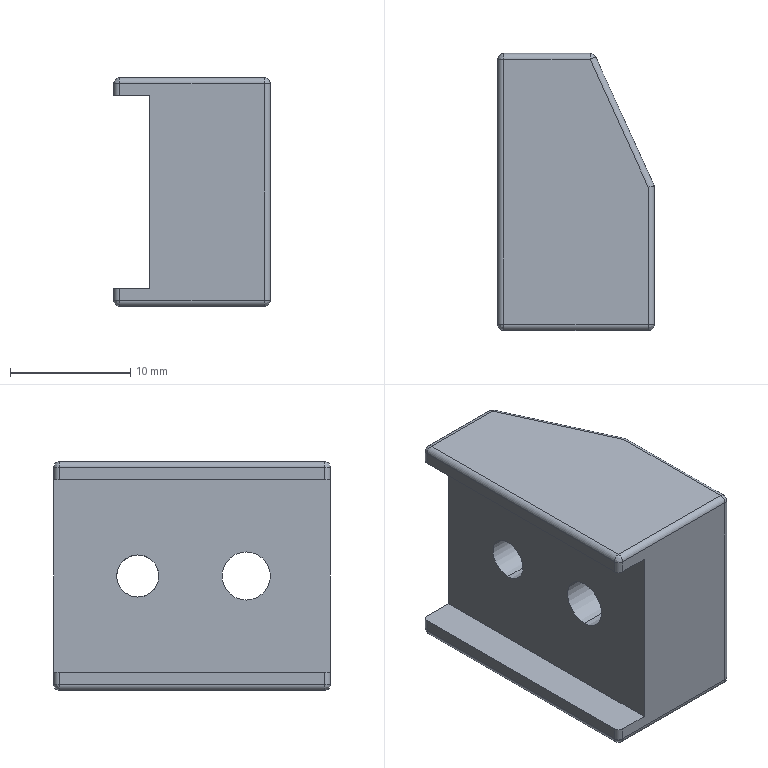Part | STEP file | Guide wheel mechanism revised.sldasm-Part-506 | 1 solid | 39 faces | box 13 x 23 x 19 mm | volume 3841 mm3 | cylinder 20 | plane 11 | spline 8 | commonest cylinder face diameters 1 x16 3.5 x2 4 x2
STEP:
#1=CARTESIAN_POINT('',(-1.818,9.,-1.75));
#2=VERTEX_POINT('',#1);
#3=CARTESIAN_POINT('',(-1.818,9.,1.75));
#4=VERTEX_POINT('',#3);
#5=CARTESIAN_POINT('',(-1.818,9.,-1.75));
#6=CARTESIAN_POINT('',(-0.2273,5.5,-1.75));
#7=CARTESIAN_POINT('',(-0.2273,5.5,1.75));
#8=CARTESIAN_POINT('',(-1.818,9.,1.75));
#9=(BOUNDED_CURVE()B_SPLINE_CURVE(3,(#5,#6,#7,#8),.UNSPECIFIED.,.F.,.F.)B_SPLINE_CURVE_WITH_KNOTS((4,4),(1.571,4.712),.UNSPECIFIED.)CURVE()GEOMETRIC_REPRESENTATION_ITEM()RATIONAL_B_SPLINE_CURVE((1.,0.3333,0.3333,1.))REPRESENTATION_ITEM(''));
#10=EDGE_CURVE('',#2,#4,#9,.T.);
#11=ORIENTED_EDGE('',*,*,#10,.F.);
#12=CARTESIAN_POINT('',(-10.,9.,-1.75));
#13=VERTEX_POINT('',#12);
#14=CARTESIAN_POINT('',(1.865,9.,-1.75));
#15=DIRECTION('',(-1.,0.,0.));
#16=VECTOR('',#15,1000.);
#17=LINE('',#14,#16);
#18=EDGE_CURVE('',#2,#13,#17,.T.);
#19=ORIENTED_EDGE('',*,*,#18,.T.);
#20=CARTESIAN_POINT('',(-10.,9.,1.75));
#21=VERTEX_POINT('',#20);
#22=CARTESIAN_POINT('',(-10.,9.,0.));
#23=DIRECTION('',(-1.,0.,0.));
#24=DIRECTION('',(0.,0.,1.));
#25=AXIS2_PLACEMENT_3D('',#22,#23,#24);
#26=CIRCLE('',#25,1.75);
#27=EDGE_CURVE('',#13,#21,#26,.T.);
#28=ORIENTED_EDGE('',*,*,#27,.T.);
#29=CARTESIAN_POINT('',(1.865,9.,1.75));
#30=DIRECTION('',(-1.,0.,0.));
#31=VECTOR('',#30,1000.);
#32=LINE('',#29,#31);
#33=EDGE_CURVE('',#4,#21,#32,.T.);
#34=ORIENTED_EDGE('',*,*,#33,.F.);
#35=EDGE_LOOP('',(#11,#19,#28,#34));
#36=FACE_OUTER_BOUND('',#35,.T.);
#37=CARTESIAN_POINT('',(1.865,9.,0.));
#38=DIRECTION('',(-1.,0.,0.));
#39=DIRECTION('',(0.,0.,1.));
#40=AXIS2_PLACEMENT_3D('',#37,#38,#39);
#41=CYLINDRICAL_SURFACE('',#40,1.75);
#42=ADVANCED_FACE('',(#36),#41,.F.);
#43=CARTESIAN_POINT('',(0.,0.,-2.));
#44=VERTEX_POINT('',#43);
#45=CARTESIAN_POINT('',(0.,0.,2.));
#46=VERTEX_POINT('',#45);
#47=CARTESIAN_POINT('',(0.,0.,0.));
#48=DIRECTION('',(-1.,0.,0.));
#49=DIRECTION('',(0.,0.,1.));
#50=AXIS2_PLACEMENT_3D('',#47,#48,#49);
#51=CIRCLE('',#50,2.);
#52=EDGE_CURVE('',#44,#46,#51,.T.);
#53=ORIENTED_EDGE('',*,*,#52,.F.);
#54=CARTESIAN_POINT('',(-10.,0.,-2.));
#55=VERTEX_POINT('',#54);
#56=CARTESIAN_POINT('',(0.,0.,-2.));
#57=DIRECTION('',(-1.,0.,0.));
#58=VECTOR('',#57,1000.);
#59=LINE('',#56,#58);
#60=EDGE_CURVE('',#44,#55,#59,.T.);
#61=ORIENTED_EDGE('',*,*,#60,.T.);
#62=CARTESIAN_POINT('',(-10.,0.,2.));
#63=VERTEX_POINT('',#62);
#64=CARTESIAN_POINT('',(-10.,0.,0.));
#65=DIRECTION('',(-1.,0.,0.));
#66=DIRECTION('',(0.,0.,1.));
#67=AXIS2_PLACEMENT_3D('',#64,#65,#66);
#68=CIRCLE('',#67,2.);
#69=EDGE_CURVE('',#55,#63,#68,.T.);
#70=ORIENTED_EDGE('',*,*,#69,.T.);
#71=CARTESIAN_POINT('',(0.,0.,2.));
#72=DIRECTION('',(-1.,0.,0.));
#73=VECTOR('',#72,1000.);
#74=LINE('',#71,#73);
#75=EDGE_CURVE('',#46,#63,#74,.T.);
#76=ORIENTED_EDGE('',*,*,#75,.F.);
#77=EDGE_LOOP('',(#53,#61,#70,#76));
#78=FACE_OUTER_BOUND('',#77,.T.);
#79=CARTESIAN_POINT('',(0.,0.,0.));
#80=DIRECTION('',(-1.,0.,0.));
#81=DIRECTION('',(0.,0.,1.));
#82=AXIS2_PLACEMENT_3D('',#79,#80,#81);
#83=CYLINDRICAL_SURFACE('',#82,2.);
#84=ADVANCED_FACE('',(#78),#83,.F.);
#85=CARTESIAN_POINT('',(-10.,9.,0.));
#86=DIRECTION('',(-1.,0.,0.));
#87=DIRECTION('',(0.,0.,1.));
#88=AXIS2_PLACEMENT_3D('',#85,#86,#87);
#89=CIRCLE('',#88,1.75);
#90=EDGE_CURVE('',#21,#13,#89,.T.);
#91=ORIENTED_EDGE('',*,*,#90,.F.);
#92=ORIENTED_EDGE('',*,*,#27,.F.);
#93=EDGE_LOOP('',(#91,#92));
#94=FACE_BOUND('',#93,.T.);
#95=CARTESIAN_POINT('',(-10.,0.,0.));
#96=DIRECTION('',(-1.,0.,0.));
#97=DIRECTION('',(0.,0.,1.));
#98=AXIS2_PLACEMENT_3D('',#95,#96,#97);
#99=CIRCLE('',#98,2.);
#100=EDGE_CURVE('',#63,#55,#99,.T.);
#101=ORIENTED_EDGE('',*,*,#100,.F.);
#102=ORIENTED_EDGE('',*,*,#69,.F.);
#103=EDGE_LOOP('',(#101,#102));
#104=FACE_BOUND('',#103,.T.);
#105=CARTESIAN_POINT('',(-10.,16.,-8.));
#106=VERTEX_POINT('',#105);
#107=CARTESIAN_POINT('',(-10.,16.,8.));
#108=VERTEX_POINT('',#107);
#109=CARTESIAN_POINT('',(-10.,16.,-8.));
#110=DIRECTION('',(0.,0.,1.));
#111=VECTOR('',#110,1000.);
#112=LINE('',#109,#111);
#113=EDGE_CURVE('',#106,#108,#112,.T.);
#114=ORIENTED_EDGE('',*,*,#113,.F.);
#115=CARTESIAN_POINT('',(-10.,-7.,-8.));
#116=VERTEX_POINT('',#115);
#117=CARTESIAN_POINT('',(-10.,-7.,-8.));
#118=DIRECTION('',(0.,1.,0.));
#119=VECTOR('',#118,1000.);
#120=LINE('',#117,#119);
#121=EDGE_CURVE('',#116,#106,#120,.T.);
#122=ORIENTED_EDGE('',*,*,#121,.F.);
#123=CARTESIAN_POINT('',(-10.,-7.,8.));
#124=VERTEX_POINT('',#123);
#125=CARTESIAN_POINT('',(-10.,-7.,-8.));
#126=DIRECTION('',(0.,0.,-1.));
#127=VECTOR('',#126,1000.);
#128=LINE('',#125,#127);
#129=EDGE_CURVE('',#124,#116,#128,.T.);
#130=ORIENTED_EDGE('',*,*,#129,.F.);
#131=CARTESIAN_POINT('',(-10.,-7.,8.));
#132=DIRECTION('',(0.,-1.,0.));
#133=VECTOR('',#132,1000.);
#134=LINE('',#131,#133);
#135=EDGE_CURVE('',#108,#124,#134,.T.);
#136=ORIENTED_EDGE('',*,*,#135,.F.);
#137=EDGE_LOOP('',(#114,#122,#130,#136));
#138=FACE_OUTER_BOUND('',#137,.T.);
#139=CARTESIAN_POINT('',(-10.,-7.,-8.));
#140=DIRECTION('',(1.,0.,0.));
#141=DIRECTION('',(0.,0.,-1.));
#142=AXIS2_PLACEMENT_3D('',#139,#140,#141);
#143=PLANE('',#142);
#144=ADVANCED_FACE('',(#94,#104,#138),#143,.F.);
#145=ORIENTED_EDGE('',*,*,#18,.F.);
#146=CARTESIAN_POINT('',(-1.818,9.,1.75));
#147=CARTESIAN_POINT('',(-3.409,12.5,1.75));
#148=CARTESIAN_POINT('',(-3.409,12.5,-1.75));
#149=CARTESIAN_POINT('',(-1.818,9.,-1.75));
#150=(BOUNDED_CURVE()B_SPLINE_CURVE(3,(#146,#147,#148,#149),.UNSPECIFIED.,.F.,.F.)B_SPLINE_CURVE_WITH_KNOTS((4,4),(4.712,7.854),.UNSPECIFIED.)CURVE()GEOMETRIC_REPRESENTATION_ITEM()RATIONAL_B_SPLINE_CURVE((1.,0.3333,0.3333,1.))REPRESENTATION_ITEM(''));
#151=EDGE_CURVE('',#4,#2,#150,.T.);
#152=ORIENTED_EDGE('',*,*,#151,.F.);
#153=ORIENTED_EDGE('',*,*,#33,.T.);
#154=ORIENTED_EDGE('',*,*,#90,.T.);
#155=EDGE_LOOP('',(#145,#152,#153,#154));
#156=FACE_OUTER_BOUND('',#155,.T.);
#157=CARTESIAN_POINT('',(1.865,9.,0.));
#158=DIRECTION('',(-1.,0.,0.));
#159=DIRECTION('',(0.,0.,1.));
#160=AXIS2_PLACEMENT_3D('',#157,#158,#159);
#161=CYLINDRICAL_SURFACE('',#160,1.75);
#162=ADVANCED_FACE('',(#156),#161,.F.);
#163=ORIENTED_EDGE('',*,*,#60,.F.);
#164=CARTESIAN_POINT('',(0.,0.,0.));
#165=DIRECTION('',(-1.,0.,0.));
#166=DIRECTION('',(0.,0.,1.));
#167=AXIS2_PLACEMENT_3D('',#164,#165,#166);
#168=CIRCLE('',#167,2.);
#169=EDGE_CURVE('',#46,#44,#168,.T.);
#170=ORIENTED_EDGE('',*,*,#169,.F.);
#171=ORIENTED_EDGE('',*,*,#75,.T.);
#172=ORIENTED_EDGE('',*,*,#100,.T.);
#173=EDGE_LOOP('',(#163,#170,#171,#172));
#174=FACE_OUTER_BOUND('',#173,.T.);
#175=CARTESIAN_POINT('',(0.,0.,0.));
#176=DIRECTION('',(-1.,0.,0.));
#177=DIRECTION('',(0.,0.,1.));
#178=AXIS2_PLACEMENT_3D('',#175,#176,#177);
#179=CYLINDRICAL_SURFACE('',#178,2.);
#180=ADVANCED_FACE('',(#174),#179,.F.);
#181=CARTESIAN_POINT('',(-12.5,16.,8.));
#182=VERTEX_POINT('',#181);
#183=CARTESIAN_POINT('',(-10.,16.,8.));
#184=DIRECTION('',(-1.,0.,0.));
#185=VECTOR('',#184,1000.);
#186=LINE('',#183,#185);
#187=EDGE_CURVE('',#108,#182,#186,.T.);
#188=ORIENTED_EDGE('',*,*,#187,.F.);
#189=ORIENTED_EDGE('',*,*,#135,.T.);
#190=CARTESIAN_POINT('',(-12.5,-7.,8.));
#191=VERTEX_POINT('',#190);
#192=CARTESIAN_POINT('',(-10.,-7.,8.));
#193=DIRECTION('',(1.,0.,0.));
#194=VECTOR('',#193,1000.);
#195=LINE('',#192,#194);
#196=EDGE_CURVE('',#191,#124,#195,.T.);
#197=ORIENTED_EDGE('',*,*,#196,.F.);
#198=CARTESIAN_POINT('',(-13.,-6.5,8.));
#199=VERTEX_POINT('',#198);
#200=CARTESIAN_POINT('',(-12.5,-6.5,8.));
#201=DIRECTION('',(0.,0.,1.));
#202=DIRECTION('',(1.,0.,0.));
#203=AXIS2_PLACEMENT_3D('',#200,#201,#202);
#204=CIRCLE('',#203,0.5);
#205=EDGE_CURVE('',#199,#191,#204,.T.);
#206=ORIENTED_EDGE('',*,*,#205,.F.);
#207=CARTESIAN_POINT('',(-13.,15.5,8.));
#208=VERTEX_POINT('',#207);
#209=CARTESIAN_POINT('',(-13.,-7.,8.));
#210=DIRECTION('',(0.,-1.,0.));
#211=VECTOR('',#210,1000.);
#212=LINE('',#209,#211);
#213=EDGE_CURVE('',#208,#199,#212,.T.);
#214=ORIENTED_EDGE('',*,*,#213,.F.);
#215=CARTESIAN_POINT('',(-12.5,15.5,8.));
#216=DIRECTION('',(0.,0.,1.));
#217=DIRECTION('',(-1.,0.,0.));
#218=AXIS2_PLACEMENT_3D('',#215,#216,#217);
#219=CIRCLE('',#218,0.5);
#220=EDGE_CURVE('',#182,#208,#219,.T.);
#221=ORIENTED_EDGE('',*,*,#220,.F.);
#222=EDGE_LOOP('',(#188,#189,#197,#206,#214,#221));
#223=FACE_OUTER_BOUND('',#222,.T.);
#224=CARTESIAN_POINT('',(-10.,-7.,8.));
#225=DIRECTION('',(0.,0.,1.));
#226=DIRECTION('',(1.,0.,0.));
#227=AXIS2_PLACEMENT_3D('',#224,#225,#226);
#228=PLANE('',#227);
#229=ADVANCED_FACE('',(#223),#228,.F.);
#230=CARTESIAN_POINT('',(-12.5,16.,-8.));
#231=VERTEX_POINT('',#230);
#232=CARTESIAN_POINT('',(0.,16.,-8.));
#233=DIRECTION('',(1.,0.,0.));
#234=VECTOR('',#233,1000.);
#235=LINE('',#232,#234);
#236=EDGE_CURVE('',#231,#106,#235,.T.);
#237=ORIENTED_EDGE('',*,*,#236,.T.);
#238=ORIENTED_EDGE('',*,*,#113,.T.);
#239=ORIENTED_EDGE('',*,*,#187,.T.);
#240=CARTESIAN_POINT('',(-12.5,16.,9.));
#241=VERTEX_POINT('',#240);
#242=CARTESIAN_POINT('',(-12.5,16.,9.5));
#243=DIRECTION('',(0.,0.,1.));
#244=VECTOR('',#243,1000.);
#245=LINE('',#242,#244);
#246=EDGE_CURVE('',#182,#241,#245,.T.);
#247=ORIENTED_EDGE('',*,*,#246,.T.);
#248=CARTESIAN_POINT('',(-5.322,16.,9.));
#249=VERTEX_POINT('',#248);
#250=CARTESIAN_POINT('',(0.,16.,9.));
#251=DIRECTION('',(1.,0.,0.));
#252=VECTOR('',#251,1000.);
#253=LINE('',#250,#252);
#254=EDGE_CURVE('',#241,#249,#253,.T.);
#255=ORIENTED_EDGE('',*,*,#254,.T.);
#256=CARTESIAN_POINT('',(-5.322,16.,-9.));
#257=VERTEX_POINT('',#256);
#258=CARTESIAN_POINT('',(-5.322,16.,9.5));
#259=DIRECTION('',(0.,0.,-1.));
#260=VECTOR('',#259,1000.);
#261=LINE('',#258,#260);
#262=EDGE_CURVE('',#249,#257,#261,.T.);
#263=ORIENTED_EDGE('',*,*,#262,.T.);
#264=CARTESIAN_POINT('',(-12.5,16.,-9.));
#265=VERTEX_POINT('',#264);
#266=CARTESIAN_POINT('',(0.,16.,-9.));
#267=DIRECTION('',(-1.,0.,0.));
#268=VECTOR('',#267,1000.);
#269=LINE('',#266,#268);
#270=EDGE_CURVE('',#257,#265,#269,.T.);
#271=ORIENTED_EDGE('',*,*,#270,.T.);
#272=CARTESIAN_POINT('',(-12.5,16.,9.5));
#273=DIRECTION('',(0.,0.,1.));
#274=VECTOR('',#273,1000.);
#275=LINE('',#272,#274);
#276=EDGE_CURVE('',#265,#231,#275,.T.);
#277=ORIENTED_EDGE('',*,*,#276,.T.);
#278=EDGE_LOOP('',(#237,#238,#239,#247,#255,#263,#271,#277));
#279=FACE_OUTER_BOUND('',#278,.T.);
#280=CARTESIAN_POINT('',(0.,16.,9.5));
#281=DIRECTION('',(0.,1.,0.));
#282=DIRECTION('',(0.,0.,1.));
#283=AXIS2_PLACEMENT_3D('',#280,#281,#282);
#284=PLANE('',#283);
#285=ADVANCED_FACE('',(#279),#284,.T.);
#286=CARTESIAN_POINT('',(-12.5,-7.,-8.));
#287=VERTEX_POINT('',#286);
#288=CARTESIAN_POINT('',(-13.,-7.,-8.));
#289=DIRECTION('',(-1.,0.,0.));
#290=VECTOR('',#289,1000.);
#291=LINE('',#288,#290);
#292=EDGE_CURVE('',#116,#287,#291,.T.);
#293=ORIENTED_EDGE('',*,*,#292,.F.);
#294=ORIENTED_EDGE('',*,*,#121,.T.);
#295=ORIENTED_EDGE('',*,*,#236,.F.);
#296=CARTESIAN_POINT('',(-13.,15.5,-8.));
#297=VERTEX_POINT('',#296);
#298=CARTESIAN_POINT('',(-12.5,15.5,-8.));
#299=DIRECTION('',(0.,0.,-1.));
#300=DIRECTION('',(-1.,0.,0.));
#301=AXIS2_PLACEMENT_3D('',#298,#299,#300);
#302=CIRCLE('',#301,0.5);
#303=EDGE_CURVE('',#297,#231,#302,.T.);
#304=ORIENTED_EDGE('',*,*,#303,.F.);
#305=CARTESIAN_POINT('',(-13.,-6.5,-8.));
#306=VERTEX_POINT('',#305);
#307=CARTESIAN_POINT('',(-13.,-7.,-8.));
#308=DIRECTION('',(0.,1.,0.));
#309=VECTOR('',#308,1000.);
#310=LINE('',#307,#309);
#311=EDGE_CURVE('',#306,#297,#310,.T.);
#312=ORIENTED_EDGE('',*,*,#311,.F.);
#313=CARTESIAN_POINT('',(-12.5,-6.5,-8.));
#314=DIRECTION('',(0.,0.,-1.));
#315=DIRECTION('',(1.,0.,0.));
#316=AXIS2_PLACEMENT_3D('',#313,#314,#315);
#317=CIRCLE('',#316,0.5);
#318=EDGE_CURVE('',#287,#306,#317,.T.);
#319=ORIENTED_EDGE('',*,*,#318,.F.);
#320=EDGE_LOOP('',(#293,#294,#295,#304,#312,#319));
#321=FACE_OUTER_BOUND('',#320,.T.);
#322=CARTESIAN_POINT('',(-13.,-7.,-8.));
#323=DIRECTION('',(0.,0.,-1.));
#324=DIRECTION('',(-1.,0.,0.));
#325=AXIS2_PLACEMENT_3D('',#322,#323,#324);
#326=PLANE('',#325);
#327=ADVANCED_FACE('',(#321),#326,.F.);
#328=ORIENTED_EDGE('',*,*,#196,.T.);
#329=ORIENTED_EDGE('',*,*,#129,.T.);
#330=ORIENTED_EDGE('',*,*,#292,.T.);
#331=CARTESIAN_POINT('',(-12.5,-7.,-9.));
#332=VERTEX_POINT('',#331);
#333=CARTESIAN_POINT('',(-12.5,-7.,-9.5));
#334=DIRECTION('',(0.,0.,-1.));
#335=VECTOR('',#334,1000.);
#336=LINE('',#333,#335);
#337=EDGE_CURVE('',#287,#332,#336,.T.);
#338=ORIENTED_EDGE('',*,*,#337,.T.);
#339=CARTESIAN_POINT('',(-0.5,-7.,-9.));
#340=VERTEX_POINT('',#339);
#341=CARTESIAN_POINT('',(0.,-7.,-9.));
#342=DIRECTION('',(1.,0.,0.));
#343=VECTOR('',#342,1000.);
#344=LINE('',#341,#343);
#345=EDGE_CURVE('',#332,#340,#344,.T.);
#346=ORIENTED_EDGE('',*,*,#345,.T.);
#347=CARTESIAN_POINT('',(-0.5,-7.,9.));
#348=VERTEX_POINT('',#347);
#349=CARTESIAN_POINT('',(-0.5,-7.,-9.5));
#350=DIRECTION('',(0.,0.,1.));
#351=VECTOR('',#350,1000.);
#352=LINE('',#349,#351);
#353=EDGE_CURVE('',#340,#348,#352,.T.);
#354=ORIENTED_EDGE('',*,*,#353,.T.);
#355=CARTESIAN_POINT('',(-12.5,-7.,9.));
#356=VERTEX_POINT('',#355);
#357=CARTESIAN_POINT('',(0.,-7.,9.));
#358=DIRECTION('',(-1.,0.,0.));
#359=VECTOR('',#358,1000.);
#360=LINE('',#357,#359);
#361=EDGE_CURVE('',#348,#356,#360,.T.);
#362=ORIENTED_EDGE('',*,*,#361,.T.);
#363=CARTESIAN_POINT('',(-12.5,-7.,-9.5));
#364=DIRECTION('',(0.,0.,-1.));
#365=VECTOR('',#364,1000.);
#366=LINE('',#363,#365);
#367=EDGE_CURVE('',#356,#191,#366,.T.);
#368=ORIENTED_EDGE('',*,*,#367,.T.);
#369=EDGE_LOOP('',(#328,#329,#330,#338,#346,#354,#362,#368));
#370=FACE_OUTER_BOUND('',#369,.T.);
#371=CARTESIAN_POINT('',(0.,-7.,-9.5));
#372=DIRECTION('',(0.,-1.,0.));
#373=DIRECTION('',(0.,0.,-1.));
#374=AXIS2_PLACEMENT_3D('',#371,#372,#373);
#375=PLANE('',#374);
#376=ADVANCED_FACE('',(#370),#375,.T.);
#377=ORIENTED_EDGE('',*,*,#151,.T.);
#378=ORIENTED_EDGE('',*,*,#10,.T.);
#379=EDGE_LOOP('',(#377,#378));
#380=FACE_BOUND('',#379,.T.);
#381=CARTESIAN_POINT('',(0.,5.,-9.));
#382=VERTEX_POINT('',#381);
#383=CARTESIAN_POINT('',(-4.867,15.707,-9.));
#384=VERTEX_POINT('',#383);
#385=CARTESIAN_POINT('',(-2.5,10.5,-9.));
#386=DIRECTION('',(-0.4138,0.9104,0.));
#387=VECTOR('',#386,1000.);
#388=LINE('',#385,#387);
#389=EDGE_CURVE('',#382,#384,#388,.T.);
#390=ORIENTED_EDGE('',*,*,#389,.T.);
#391=CARTESIAN_POINT('',(-4.867,15.707,9.));
#392=VERTEX_POINT('',#391);
#393=CARTESIAN_POINT('',(-4.867,15.707,0.));
#394=DIRECTION('',(0.,0.,1.));
#395=VECTOR('',#394,1000.);
#396=LINE('',#393,#395);
#397=EDGE_CURVE('',#384,#392,#396,.T.);
#398=ORIENTED_EDGE('',*,*,#397,.T.);
#399=CARTESIAN_POINT('',(0.,5.,9.));
#400=VERTEX_POINT('',#399);
#401=CARTESIAN_POINT('',(-2.5,10.5,9.));
#402=DIRECTION('',(0.4138,-0.9104,0.));
#403=VECTOR('',#402,1000.);
#404=LINE('',#401,#403);
#405=EDGE_CURVE('',#392,#400,#404,.T.);
#406=ORIENTED_EDGE('',*,*,#405,.T.);
#407=CARTESIAN_POINT('',(0.,5.,0.));
#408=DIRECTION('',(0.,0.,-1.));
#409=VECTOR('',#408,1000.);
#410=LINE('',#407,#409);
#411=EDGE_CURVE('',#400,#382,#410,.T.);
#412=ORIENTED_EDGE('',*,*,#411,.T.);
#413=EDGE_LOOP('',(#390,#398,#406,#412));
#414=FACE_OUTER_BOUND('',#413,.T.);
#415=CARTESIAN_POINT('',(-2.5,10.5,0.));
#416=DIRECTION('',(0.9104,0.4138,0.));
#417=DIRECTION('',(-0.4138,0.9104,0.));
#418=AXIS2_PLACEMENT_3D('',#415,#416,#417);
#419=PLANE('',#418);
#420=ADVANCED_FACE('',(#380,#414),#419,.T.);
#421=ORIENTED_EDGE('',*,*,#169,.T.);
#422=ORIENTED_EDGE('',*,*,#52,.T.);
#423=EDGE_LOOP('',(#421,#422));
#424=FACE_BOUND('',#423,.T.);
#425=CARTESIAN_POINT('',(0.,-6.5,9.));
#426=VERTEX_POINT('',#425);
#427=CARTESIAN_POINT('',(0.,0.,9.));
#428=DIRECTION('',(0.,1.,0.));
#429=VECTOR('',#428,1000.);
#430=LINE('',#427,#429);
#431=EDGE_CURVE('',#426,#400,#430,.T.);
#432=ORIENTED_EDGE('',*,*,#431,.F.);
#433=CARTESIAN_POINT('',(0.,-6.5,-9.));
#434=VERTEX_POINT('',#433);
#435=CARTESIAN_POINT('',(0.,-6.5,0.));
#436=DIRECTION('',(0.,0.,1.));
#437=VECTOR('',#436,1000.);
#438=LINE('',#435,#437);
#439=EDGE_CURVE('',#434,#426,#438,.T.);
#440=ORIENTED_EDGE('',*,*,#439,.F.);
#441=CARTESIAN_POINT('',(0.,0.,-9.));
#442=DIRECTION('',(0.,-1.,0.));
#443=VECTOR('',#442,1000.);
#444=LINE('',#441,#443);
#445=EDGE_CURVE('',#382,#434,#444,.T.);
#446=ORIENTED_EDGE('',*,*,#445,.F.);
#447=ORIENTED_EDGE('',*,*,#411,.F.);
#448=EDGE_LOOP('',(#432,#440,#446,#447));
#449=FACE_OUTER_BOUND('',#448,.T.);
#450=CARTESIAN_POINT('',(0.,0.,0.));
#451=DIRECTION('',(-1.,0.,0.));
#452=DIRECTION('',(0.,0.,1.));
#453=AXIS2_PLACEMENT_3D('',#450,#451,#452);
#454=PLANE('',#453);
#455=ADVANCED_FACE('',(#424,#449),#454,.F.);
#456=ORIENTED_EDGE('',*,*,#246,.F.);
#457=ORIENTED_EDGE('',*,*,#220,.T.);
#458=CARTESIAN_POINT('',(-13.,15.5,9.));
#459=VERTEX_POINT('',#458);
#460=CARTESIAN_POINT('',(-13.,15.5,9.504));
#461=DIRECTION('',(0.,0.,1.));
#462=VECTOR('',#461,1000.);
#463=LINE('',#460,#462);
#464=EDGE_CURVE('',#208,#459,#463,.T.);
#465=ORIENTED_EDGE('',*,*,#464,.T.);
#466=CARTESIAN_POINT('',(-12.5,15.5,9.));
#467=DIRECTION('',(0.,0.,-1.));
#468=DIRECTION('',(-1.,0.,0.));
#469=AXIS2_PLACEMENT_3D('',#466,#467,#468);
#470=CIRCLE('',#469,0.5);
#471=EDGE_CURVE('',#459,#241,#470,.T.);
#472=ORIENTED_EDGE('',*,*,#471,.T.);
#473=EDGE_LOOP('',(#456,#457,#465,#472));
#474=FACE_OUTER_BOUND('',#473,.T.);
#475=CARTESIAN_POINT('',(-12.5,15.5,9.504));
#476=DIRECTION('',(0.,0.,-1.));
#477=DIRECTION('',(-1.,0.,0.));
#478=AXIS2_PLACEMENT_3D('',#475,#476,#477);
#479=CYLINDRICAL_SURFACE('',#478,0.5);
#480=ADVANCED_FACE('',(#474),#479,.T.);
#481=CARTESIAN_POINT('',(-13.,-6.5,9.));
#482=VERTEX_POINT('',#481);
#483=CARTESIAN_POINT('',(-13.,-6.5,-9.504));
#484=DIRECTION('',(0.,0.,-1.));
#485=VECTOR('',#484,1000.);
#486=LINE('',#483,#485);
#487=EDGE_CURVE('',#482,#199,#486,.T.);
#488=ORIENTED_EDGE('',*,*,#487,.T.);
#489=ORIENTED_EDGE('',*,*,#205,.T.);
#490=ORIENTED_EDGE('',*,*,#367,.F.);
#491=CARTESIAN_POINT('',(-12.5,-6.5,9.));
#492=DIRECTION('',(0.,0.,-1.));
#493=DIRECTION('',(1.,0.,0.));
#494=AXIS2_PLACEMENT_3D('',#491,#492,#493);
#495=CIRCLE('',#494,0.5);
#496=EDGE_CURVE('',#356,#482,#495,.T.);
#497=ORIENTED_EDGE('',*,*,#496,.T.);
#498=EDGE_LOOP('',(#488,#489,#490,#497));
#499=FACE_OUTER_BOUND('',#498,.T.);
#500=CARTESIAN_POINT('',(-12.5,-6.5,-9.504));
#501=DIRECTION('',(0.,0.,1.));
#502=DIRECTION('',(1.,0.,0.));
#503=AXIS2_PLACEMENT_3D('',#500,#501,#502);
#504=CYLINDRICAL_SURFACE('',#503,0.5);
#505=ADVANCED_FACE('',(#499),#504,.T.);
#506=ORIENTED_EDGE('',*,*,#464,.F.);
#507=ORIENTED_EDGE('',*,*,#213,.T.);
#508=ORIENTED_EDGE('',*,*,#487,.F.);
#509=CARTESIAN_POINT('',(-13.,0.,9.));
#510=DIRECTION('',(0.,1.,0.));
#511=VECTOR('',#510,1000.);
#512=LINE('',#509,#511);
#513=EDGE_CURVE('',#482,#459,#512,.T.);
#514=ORIENTED_EDGE('',*,*,#513,.T.);
#515=EDGE_LOOP('',(#506,#507,#508,#514));
#516=FACE_OUTER_BOUND('',#515,.T.);
#517=CARTESIAN_POINT('',(-13.,0.,0.));
#518=DIRECTION('',(-1.,0.,0.));
#519=DIRECTION('',(0.,0.,1.));
#520=AXIS2_PLACEMENT_3D('',#517,#518,#519);
#521=PLANE('',#520);
#522=ADVANCED_FACE('',(#516),#521,.T.);
#523=CARTESIAN_POINT('',(-13.,15.5,-9.));
#524=VERTEX_POINT('',#523);
#525=CARTESIAN_POINT('',(-13.,15.5,9.504));
#526=DIRECTION('',(0.,0.,1.));
#527=VECTOR('',#526,1000.);
#528=LINE('',#525,#527);
#529=EDGE_CURVE('',#524,#297,#528,.T.);
#530=ORIENTED_EDGE('',*,*,#529,.T.);
#531=ORIENTED_EDGE('',*,*,#303,.T.);
#532=ORIENTED_EDGE('',*,*,#276,.F.);
#533=CARTESIAN_POINT('',(-12.5,15.5,-9.));
#534=DIRECTION('',(0.,0.,1.));
#535=DIRECTION('',(-1.,0.,0.));
#536=AXIS2_PLACEMENT_3D('',#533,#534,#535);
#537=CIRCLE('',#536,0.5);
#538=EDGE_CURVE('',#265,#524,#537,.T.);
#539=ORIENTED_EDGE('',*,*,#538,.T.);
#540=EDGE_LOOP('',(#530,#531,#532,#539));
#541=FACE_OUTER_BOUND('',#540,.T.);
#542=CARTESIAN_POINT('',(-12.5,15.5,9.504));
#543=DIRECTION('',(0.,0.,-1.));
#544=DIRECTION('',(-1.,0.,0.));
#545=AXIS2_PLACEMENT_3D('',#542,#543,#544);
#546=CYLINDRICAL_SURFACE('',#545,0.5);
#547=ADVANCED_FACE('',(#541),#546,.T.);
#548=CARTESIAN_POINT('',(-12.5,15.5,-9.5));
#549=VERTEX_POINT('',#548);
#550=CARTESIAN_POINT('',(-12.5,15.5,-9.));
#551=DIRECTION('',(1.,0.,0.));
#552=DIRECTION('',(0.,0.,-1.));
#553=AXIS2_PLACEMENT_3D('',#550,#551,#552);
#554=CIRCLE('',#553,0.5);
#555=EDGE_CURVE('',#549,#265,#554,.T.);
#556=ORIENTED_EDGE('',*,*,#555,.T.);
#557=ORIENTED_EDGE('',*,*,#270,.F.);
#558=CARTESIAN_POINT('',(-5.322,15.5,-9.5));
#559=VERTEX_POINT('',#558);
#560=CARTESIAN_POINT('',(-5.322,15.5,-9.));
#561=DIRECTION('',(-1.,0.,0.));
#562=DIRECTION('',(0.,0.,-1.));
#563=AXIS2_PLACEMENT_3D('',#560,#561,#562);
#564=CIRCLE('',#563,0.5);
#565=EDGE_CURVE('',#257,#559,#564,.T.);
#566=ORIENTED_EDGE('',*,*,#565,.T.);
#567=CARTESIAN_POINT('',(-13.024,15.5,-9.5));
#568=DIRECTION('',(-1.,0.,0.));
#569=VECTOR('',#568,1000.);
#570=LINE('',#567,#569);
#571=EDGE_CURVE('',#559,#549,#570,.T.);
#572=ORIENTED_EDGE('',*,*,#571,.T.);
#573=EDGE_LOOP('',(#556,#557,#566,#572));
#574=FACE_OUTER_BOUND('',#573,.T.);
#575=CARTESIAN_POINT('',(-13.024,15.5,-9.));
#576=DIRECTION('',(1.,0.,0.));
#577=DIRECTION('',(0.,0.,-1.));
#578=AXIS2_PLACEMENT_3D('',#575,#576,#577);
#579=CYLINDRICAL_SURFACE('',#578,0.5);
#580=ADVANCED_FACE('',(#574),#579,.T.);
#581=CARTESIAN_POINT('',(-5.322,15.5,9.));
#582=DIRECTION('',(0.,0.,-1.));
#583=DIRECTION('',(-1.,0.,0.));
#584=AXIS2_PLACEMENT_3D('',#581,#582,#583);
#585=CIRCLE('',#584,0.5);
#586=EDGE_CURVE('',#249,#392,#585,.T.);
#587=ORIENTED_EDGE('',*,*,#586,.T.);
#588=ORIENTED_EDGE('',*,*,#397,.F.);
#589=CARTESIAN_POINT('',(-5.322,15.5,-9.));
#590=DIRECTION('',(0.,0.,1.));
#591=DIRECTION('',(-1.,0.,0.));
#592=AXIS2_PLACEMENT_3D('',#589,#590,#591);
#593=CIRCLE('',#592,0.5);
#594=EDGE_CURVE('',#384,#257,#593,.T.);
#595=ORIENTED_EDGE('',*,*,#594,.T.);
#596=ORIENTED_EDGE('',*,*,#262,.F.);
#597=EDGE_LOOP('',(#587,#588,#595,#596));
#598=FACE_OUTER_BOUND('',#597,.T.);
#599=CARTESIAN_POINT('',(-5.322,15.5,9.504));
#600=DIRECTION('',(0.,0.,-1.));
#601=DIRECTION('',(-1.,0.,0.));
#602=AXIS2_PLACEMENT_3D('',#599,#600,#601);
#603=CYLINDRICAL_SURFACE('',#602,0.5);
#604=ADVANCED_FACE('',(#598),#603,.T.);
#605=CARTESIAN_POINT('',(-12.5,15.5,9.5));
#606=VERTEX_POINT('',#605);
#607=CARTESIAN_POINT('',(-12.5,15.5,9.));
#608=DIRECTION('',(1.,0.,0.));
#609=DIRECTION('',(0.,0.,-1.));
#610=AXIS2_PLACEMENT_3D('',#607,#608,#609);
#611=CIRCLE('',#610,0.5);
#612=EDGE_CURVE('',#241,#606,#611,.T.);
#613=ORIENTED_EDGE('',*,*,#612,.T.);
#614=CARTESIAN_POINT('',(-5.322,15.5,9.5));
#615=VERTEX_POINT('',#614);
#616=CARTESIAN_POINT('',(-13.019,15.5,9.5));
#617=DIRECTION('',(1.,0.,0.));
#618=VECTOR('',#617,1000.);
#619=LINE('',#616,#618);
#620=EDGE_CURVE('',#606,#615,#619,.T.);
#621=ORIENTED_EDGE('',*,*,#620,.T.);
#622=CARTESIAN_POINT('',(-5.322,15.5,9.));
#623=DIRECTION('',(-1.,0.,0.));
#624=DIRECTION('',(0.,0.,-1.));
#625=AXIS2_PLACEMENT_3D('',#622,#623,#624);
#626=CIRCLE('',#625,0.5);
#627=EDGE_CURVE('',#615,#249,#626,.T.);
#628=ORIENTED_EDGE('',*,*,#627,.T.);
#629=ORIENTED_EDGE('',*,*,#254,.F.);
#630=EDGE_LOOP('',(#613,#621,#628,#629));
#631=FACE_OUTER_BOUND('',#630,.T.);
#632=CARTESIAN_POINT('',(-13.019,15.5,9.));
#633=DIRECTION('',(1.,0.,0.));
#634=DIRECTION('',(0.,0.,-1.));
#635=AXIS2_PLACEMENT_3D('',#632,#633,#634);
#636=CYLINDRICAL_SURFACE('',#635,0.5);
#637=ADVANCED_FACE('',(#631),#636,.T.);
#638=ORIENTED_EDGE('',*,*,#337,.F.);
#639=ORIENTED_EDGE('',*,*,#318,.T.);
#640=CARTESIAN_POINT('',(-13.,-6.5,-9.));
#641=VERTEX_POINT('',#640);
#642=CARTESIAN_POINT('',(-13.,-6.5,-9.504));
#643=DIRECTION('',(0.,0.,-1.));
#644=VECTOR('',#643,1000.);
#645=LINE('',#642,#644);
#646=EDGE_CURVE('',#306,#641,#645,.T.);
#647=ORIENTED_EDGE('',*,*,#646,.T.);
#648=CARTESIAN_POINT('',(-12.5,-6.5,-9.));
#649=DIRECTION('',(0.,0.,1.));
#650=DIRECTION('',(1.,0.,0.));
#651=AXIS2_PLACEMENT_3D('',#648,#649,#650);
#652=CIRCLE('',#651,0.5);
#653=EDGE_CURVE('',#641,#332,#652,.T.);
#654=ORIENTED_EDGE('',*,*,#653,.T.);
#655=EDGE_LOOP('',(#638,#639,#647,#654));
#656=FACE_OUTER_BOUND('',#655,.T.);
#657=CARTESIAN_POINT('',(-12.5,-6.5,-9.504));
#658=DIRECTION('',(0.,0.,1.));
#659=DIRECTION('',(1.,0.,0.));
#660=AXIS2_PLACEMENT_3D('',#657,#658,#659);
#661=CYLINDRICAL_SURFACE('',#660,0.5);
#662=ADVANCED_FACE('',(#656),#661,.T.);
#663=ORIENTED_EDGE('',*,*,#646,.F.);
#664=ORIENTED_EDGE('',*,*,#311,.T.);
#665=ORIENTED_EDGE('',*,*,#529,.F.);
#666=CARTESIAN_POINT('',(-13.,0.,-9.));
#667=DIRECTION('',(0.,-1.,0.));
#668=VECTOR('',#667,1000.);
#669=LINE('',#666,#668);
#670=EDGE_CURVE('',#524,#641,#669,.T.);
#671=ORIENTED_EDGE('',*,*,#670,.T.);
#672=EDGE_LOOP('',(#663,#664,#665,#671));
#673=FACE_OUTER_BOUND('',#672,.T.);
#674=CARTESIAN_POINT('',(-13.,0.,0.));
#675=DIRECTION('',(-1.,0.,0.));
#676=DIRECTION('',(0.,0.,1.));
#677=AXIS2_PLACEMENT_3D('',#674,#675,#676);
#678=PLANE('',#677);
#679=ADVANCED_FACE('',(#673),#678,.T.);
#680=CARTESIAN_POINT('',(-0.5,-6.5,9.5));
#681=VERTEX_POINT('',#680);
#682=CARTESIAN_POINT('',(-0.5,-6.5,9.));
#683=DIRECTION('',(-1.,0.,0.));
#684=DIRECTION('',(0.,0.,-1.));
#685=AXIS2_PLACEMENT_3D('',#682,#683,#684);
#686=CIRCLE('',#685,0.5);
#687=EDGE_CURVE('',#348,#681,#686,.T.);
#688=ORIENTED_EDGE('',*,*,#687,.T.);
#689=CARTESIAN_POINT('',(-12.5,-6.5,9.5));
#690=VERTEX_POINT('',#689);
#691=CARTESIAN_POINT('',(-13.004,-6.5,9.5));
#692=DIRECTION('',(-1.,0.,0.));
#693=VECTOR('',#692,1000.);
#694=LINE('',#691,#693);
#695=EDGE_CURVE('',#681,#690,#694,.T.);
#696=ORIENTED_EDGE('',*,*,#695,.T.);
#697=CARTESIAN_POINT('',(-12.5,-6.5,9.));
#698=DIRECTION('',(1.,0.,0.));
#699=DIRECTION('',(0.,0.,-1.));
#700=AXIS2_PLACEMENT_3D('',#697,#698,#699);
#701=CIRCLE('',#700,0.5);
#702=EDGE_CURVE('',#690,#356,#701,.T.);
#703=ORIENTED_EDGE('',*,*,#702,.T.);
#704=ORIENTED_EDGE('',*,*,#361,.F.);
#705=EDGE_LOOP('',(#688,#696,#703,#704));
#706=FACE_OUTER_BOUND('',#705,.T.);
#707=CARTESIAN_POINT('',(-13.004,-6.5,9.));
#708=DIRECTION('',(1.,0.,0.));
#709=DIRECTION('',(0.,0.,-1.));
#710=AXIS2_PLACEMENT_3D('',#707,#708,#709);
#711=CYLINDRICAL_SURFACE('',#710,0.5);
#712=ADVANCED_FACE('',(#706),#711,.T.);
#713=CARTESIAN_POINT('',(-0.5,-6.5,-9.));
#714=DIRECTION('',(0.,0.,1.));
#715=DIRECTION('',(-1.,0.,0.));
#716=AXIS2_PLACEMENT_3D('',#713,#714,#715);
#717=CIRCLE('',#716,0.5);
#718=EDGE_CURVE('',#340,#434,#717,.T.);
#719=ORIENTED_EDGE('',*,*,#718,.T.);
#720=ORIENTED_EDGE('',*,*,#439,.T.);
#721=CARTESIAN_POINT('',(-0.5,-6.5,9.));
#722=DIRECTION('',(0.,0.,-1.));
#723=DIRECTION('',(-1.,0.,0.));
#724=AXIS2_PLACEMENT_3D('',#721,#722,#723);
#725=CIRCLE('',#724,0.5);
#726=EDGE_CURVE('',#426,#348,#725,.T.);
#727=ORIENTED_EDGE('',*,*,#726,.T.);
#728=ORIENTED_EDGE('',*,*,#353,.F.);
#729=EDGE_LOOP('',(#719,#720,#727,#728));
#730=FACE_OUTER_BOUND('',#729,.T.);
#731=CARTESIAN_POINT('',(-0.5,-6.5,9.504));
#732=DIRECTION('',(0.,0.,-1.));
#733=DIRECTION('',(-1.,0.,0.));
#734=AXIS2_PLACEMENT_3D('',#731,#732,#733);
#735=CYLINDRICAL_SURFACE('',#734,0.5);
#736=ADVANCED_FACE('',(#730),#735,.T.);
#737=CARTESIAN_POINT('',(-0.5,-6.5,-9.5));
#738=VERTEX_POINT('',#737);
#739=CARTESIAN_POINT('',(-0.5,-6.5,-9.));
#740=DIRECTION('',(-1.,0.,0.));
#741=DIRECTION('',(0.,0.,-1.));
#742=AXIS2_PLACEMENT_3D('',#739,#740,#741);
#743=CIRCLE('',#742,0.5);
#744=EDGE_CURVE('',#738,#340,#743,.T.);
#745=ORIENTED_EDGE('',*,*,#744,.T.);
#746=ORIENTED_EDGE('',*,*,#345,.F.);
#747=CARTESIAN_POINT('',(-12.5,-6.5,-9.5));
#748=VERTEX_POINT('',#747);
#749=CARTESIAN_POINT('',(-12.5,-6.5,-9.));
#750=DIRECTION('',(1.,0.,0.));
#751=DIRECTION('',(0.,0.,-1.));
#752=AXIS2_PLACEMENT_3D('',#749,#750,#751);
#753=CIRCLE('',#752,0.5);
#754=EDGE_CURVE('',#332,#748,#753,.T.);
#755=ORIENTED_EDGE('',*,*,#754,.T.);
#756=CARTESIAN_POINT('',(-13.004,-6.5,-9.5));
#757=DIRECTION('',(1.,0.,0.));
#758=VECTOR('',#757,1000.);
#759=LINE('',#756,#758);
#760=EDGE_CURVE('',#748,#738,#759,.T.);
#761=ORIENTED_EDGE('',*,*,#760,.T.);
#762=EDGE_LOOP('',(#745,#746,#755,#761));
#763=FACE_OUTER_BOUND('',#762,.T.);
#764=CARTESIAN_POINT('',(-13.004,-6.5,-9.));
#765=DIRECTION('',(1.,0.,0.));
#766=DIRECTION('',(0.,0.,-1.));
#767=AXIS2_PLACEMENT_3D('',#764,#765,#766);
#768=CYLINDRICAL_SURFACE('',#767,0.5);
#769=ADVANCED_FACE('',(#763),#768,.T.);
#770=CARTESIAN_POINT('',(-0.5,4.892,-9.5));
#771=VERTEX_POINT('',#770);
#772=CARTESIAN_POINT('',(0.,5.,-9.));
#773=CARTESIAN_POINT('',(0.,5.,-9.293));
#774=CARTESIAN_POINT('',(-0.2071,4.955,-9.5));
#775=CARTESIAN_POINT('',(-0.5,4.892,-9.5));
#776=(BOUNDED_CURVE()B_SPLINE_CURVE(3,(#772,#773,#774,#775),.UNSPECIFIED.,.F.,.F.)B_SPLINE_CURVE_WITH_KNOTS((4,4),(0.,1.571),.UNSPECIFIED.)CURVE()GEOMETRIC_REPRESENTATION_ITEM()RATIONAL_B_SPLINE_CURVE((1.,0.8047,0.8047,1.))REPRESENTATION_ITEM(''));
#777=EDGE_CURVE('',#382,#771,#776,.T.);
#778=ORIENTED_EDGE('',*,*,#777,.T.);
#779=CARTESIAN_POINT('',(-5.562,16.029,-9.5));
#780=DIRECTION('',(-0.4138,0.9104,0.));
#781=VECTOR('',#780,1000.);
#782=LINE('',#779,#781);
#783=EDGE_CURVE('',#771,#559,#782,.T.);
#784=ORIENTED_EDGE('',*,*,#783,.T.);
#785=CARTESIAN_POINT('',(-5.322,15.5,-9.));
#786=DIRECTION('',(0.4138,-0.9104,0.));
#787=DIRECTION('',(0.9104,0.4138,0.));
#788=AXIS2_PLACEMENT_3D('',#785,#786,#787);
#789=CIRCLE('',#788,0.5);
#790=EDGE_CURVE('',#559,#384,#789,.T.);
#791=ORIENTED_EDGE('',*,*,#790,.T.);
#792=ORIENTED_EDGE('',*,*,#389,.F.);
#793=EDGE_LOOP('',(#778,#784,#791,#792));
#794=FACE_OUTER_BOUND('',#793,.T.);
#795=CARTESIAN_POINT('',(-5.562,16.029,-9.));
#796=DIRECTION('',(0.4138,-0.9104,0.));
#797=DIRECTION('',(0.9104,0.4138,0.));
#798=AXIS2_PLACEMENT_3D('',#795,#796,#797);
#799=CYLINDRICAL_SURFACE('',#798,0.5);
#800=ADVANCED_FACE('',(#794),#799,.T.);
#801=CARTESIAN_POINT('',(-0.5,4.892,9.5));
#802=VERTEX_POINT('',#801);
#803=CARTESIAN_POINT('',(-0.5,4.892,9.5));
#804=CARTESIAN_POINT('',(-0.2071,4.955,9.5));
#805=CARTESIAN_POINT('',(0.,5.,9.293));
#806=CARTESIAN_POINT('',(0.,5.,9.));
#807=(BOUNDED_CURVE()B_SPLINE_CURVE(3,(#803,#804,#805,#806),.UNSPECIFIED.,.F.,.F.)B_SPLINE_CURVE_WITH_KNOTS((4,4),(1.571,3.142),.UNSPECIFIED.)CURVE()GEOMETRIC_REPRESENTATION_ITEM()RATIONAL_B_SPLINE_CURVE((1.,0.8047,0.8047,1.))REPRESENTATION_ITEM(''));
#808=EDGE_CURVE('',#802,#400,#807,.T.);
#809=ORIENTED_EDGE('',*,*,#808,.T.);
#810=ORIENTED_EDGE('',*,*,#405,.F.);
#811=CARTESIAN_POINT('',(-5.322,15.5,9.));
#812=DIRECTION('',(0.4138,-0.9104,0.));
#813=DIRECTION('',(-0.9104,-0.4138,0.));
#814=AXIS2_PLACEMENT_3D('',#811,#812,#813);
#815=CIRCLE('',#814,0.5);
#816=EDGE_CURVE('',#392,#615,#815,.T.);
#817=ORIENTED_EDGE('',*,*,#816,.T.);
#818=CARTESIAN_POINT('',(0.01844,3.751,9.5));
#819=DIRECTION('',(0.4138,-0.9104,0.));
#820=VECTOR('',#819,1000.);
#821=LINE('',#818,#820);
#822=EDGE_CURVE('',#615,#802,#821,.T.);
#823=ORIENTED_EDGE('',*,*,#822,.T.);
#824=EDGE_LOOP('',(#809,#810,#817,#823));
#825=FACE_OUTER_BOUND('',#824,.T.);
#826=CARTESIAN_POINT('',(0.01844,3.751,9.));
#827=DIRECTION('',(-0.4138,0.9104,0.));
#828=DIRECTION('',(-0.9104,-0.4138,0.));
#829=AXIS2_PLACEMENT_3D('',#826,#827,#828);
#830=CYLINDRICAL_SURFACE('',#829,0.5);
#831=ADVANCED_FACE('',(#825),#830,.T.);
#832=CARTESIAN_POINT('',(-0.5,-6.5,9.));
#833=DIRECTION('',(0.,1.,0.));
#834=DIRECTION('',(0.,0.,-1.));
#835=AXIS2_PLACEMENT_3D('',#832,#833,#834);
#836=CIRCLE('',#835,0.5);
#837=EDGE_CURVE('',#681,#426,#836,.T.);
#838=ORIENTED_EDGE('',*,*,#837,.T.);
#839=ORIENTED_EDGE('',*,*,#431,.T.);
#840=ORIENTED_EDGE('',*,*,#808,.F.);
#841=CARTESIAN_POINT('',(-0.5,16.034,9.5));
#842=DIRECTION('',(0.,-1.,0.));
#843=VECTOR('',#842,1000.);
#844=LINE('',#841,#843);
#845=EDGE_CURVE('',#802,#681,#844,.T.);
#846=ORIENTED_EDGE('',*,*,#845,.T.);
#847=EDGE_LOOP('',(#838,#839,#840,#846));
#848=FACE_OUTER_BOUND('',#847,.T.);
#849=CARTESIAN_POINT('',(-0.5,16.034,9.));
#850=DIRECTION('',(0.,-1.,0.));
#851=DIRECTION('',(0.,0.,-1.));
#852=AXIS2_PLACEMENT_3D('',#849,#850,#851);
#853=CYLINDRICAL_SURFACE('',#852,0.5);
#854=ADVANCED_FACE('',(#848),#853,.T.);
#855=CARTESIAN_POINT('',(-0.5,-6.5,-9.));
#856=DIRECTION('',(0.,1.,0.));
#857=DIRECTION('',(0.,0.,1.));
#858=AXIS2_PLACEMENT_3D('',#855,#856,#857);
#859=CIRCLE('',#858,0.5);
#860=EDGE_CURVE('',#434,#738,#859,.T.);
#861=ORIENTED_EDGE('',*,*,#860,.T.);
#862=CARTESIAN_POINT('',(-0.5,-7.034,-9.5));
#863=DIRECTION('',(0.,1.,0.));
#864=VECTOR('',#863,1000.);
#865=LINE('',#862,#864);
#866=EDGE_CURVE('',#738,#771,#865,.T.);
#867=ORIENTED_EDGE('',*,*,#866,.T.);
#868=ORIENTED_EDGE('',*,*,#777,.F.);
#869=ORIENTED_EDGE('',*,*,#445,.T.);
#870=EDGE_LOOP('',(#861,#867,#868,#869));
#871=FACE_OUTER_BOUND('',#870,.T.);
#872=CARTESIAN_POINT('',(-0.5,-7.034,-9.));
#873=DIRECTION('',(0.,1.,0.));
#874=DIRECTION('',(0.,0.,1.));
#875=AXIS2_PLACEMENT_3D('',#872,#873,#874);
#876=CYLINDRICAL_SURFACE('',#875,0.5);
#877=ADVANCED_FACE('',(#871),#876,.T.);
#878=ORIENTED_EDGE('',*,*,#612,.F.);
#879=ORIENTED_EDGE('',*,*,#471,.F.);
#880=CARTESIAN_POINT('',(-12.5,15.5,9.));
#881=DIRECTION('',(0.,1.,0.));
#882=DIRECTION('',(0.,0.,1.));
#883=AXIS2_PLACEMENT_3D('',#880,#881,#882);
#884=CIRCLE('',#883,0.5);
#885=EDGE_CURVE('',#459,#606,#884,.T.);
#886=ORIENTED_EDGE('',*,*,#885,.T.);
#887=EDGE_LOOP('',(#878,#879,#886));
#888=FACE_OUTER_BOUND('',#887,.T.);
#889=CARTESIAN_POINT('',(-12.495,16.,9.));
#890=CARTESIAN_POINT('',(-12.495,16.,9.207));
#891=CARTESIAN_POINT('',(-12.391,15.896,9.352));
#892=CARTESIAN_POINT('',(-12.245,15.75,9.35));
#893=CARTESIAN_POINT('',(-12.793,16.003,9.));
#894=CARTESIAN_POINT('',(-12.793,16.003,9.332));
#895=CARTESIAN_POINT('',(-12.626,15.836,9.565));
#896=CARTESIAN_POINT('',(-12.391,15.601,9.562));
#897=CARTESIAN_POINT('',(-13.003,15.793,9.));
#898=CARTESIAN_POINT('',(-13.003,15.793,9.332));
#899=CARTESIAN_POINT('',(-12.836,15.626,9.565));
#900=CARTESIAN_POINT('',(-12.601,15.391,9.562));
#901=CARTESIAN_POINT('',(-13.,15.495,9.));
#902=CARTESIAN_POINT('',(-13.,15.495,9.207));
#903=CARTESIAN_POINT('',(-12.896,15.391,9.352));
#904=CARTESIAN_POINT('',(-12.75,15.245,9.35));
#905=(BOUNDED_SURFACE()B_SPLINE_SURFACE(3,3,((#889,#890,#891,#892),(#893,#894,#895,#896),(#897,#898,#899,#900),(#901,#902,#903,#904)),.UNSPECIFIED.,.F.,.F.,.F.)B_SPLINE_SURFACE_WITH_KNOTS((4,4),(4,4),(0.,1.),(0.,1.),.UNSPECIFIED.)GEOMETRIC_REPRESENTATION_ITEM()RATIONAL_B_SPLINE_SURFACE(((1.,0.8025,0.8025,1.),(0.8003,0.6422,0.6422,0.8003),(0.8003,0.6422,0.6422,0.8003),(1.,0.8025,0.8025,1.)))REPRESENTATION_ITEM('')SURFACE());
#906=ADVANCED_FACE('',(#888),#905,.T.);
#907=ORIENTED_EDGE('',*,*,#496,.F.);
#908=ORIENTED_EDGE('',*,*,#702,.F.);
#909=CARTESIAN_POINT('',(-12.5,-6.5,9.));
#910=DIRECTION('',(0.,-1.,0.));
#911=DIRECTION('',(-0.7071,0.,0.7071));
#912=AXIS2_PLACEMENT_3D('',#909,#910,#911);
#913=CIRCLE('',#912,0.5);
#914=EDGE_CURVE('',#690,#482,#913,.T.);
#915=ORIENTED_EDGE('',*,*,#914,.T.);
#916=EDGE_LOOP('',(#907,#908,#915));
#917=FACE_OUTER_BOUND('',#916,.T.);
#918=CARTESIAN_POINT('',(-12.495,-6.5,9.5));
#919=CARTESIAN_POINT('',(-12.495,-6.707,9.5));
#920=CARTESIAN_POINT('',(-12.391,-6.852,9.396));
#921=CARTESIAN_POINT('',(-12.245,-6.85,9.25));
#922=CARTESIAN_POINT('',(-12.793,-6.5,9.503));
#923=CARTESIAN_POINT('',(-12.793,-6.832,9.503));
#924=CARTESIAN_POINT('',(-12.626,-7.065,9.336));
#925=CARTESIAN_POINT('',(-12.391,-7.062,9.101));
#926=CARTESIAN_POINT('',(-13.003,-6.5,9.293));
#927=CARTESIAN_POINT('',(-13.003,-6.832,9.293));
#928=CARTESIAN_POINT('',(-12.836,-7.065,9.126));
#929=CARTESIAN_POINT('',(-12.601,-7.062,8.891));
#930=CARTESIAN_POINT('',(-13.,-6.5,8.995));
#931=CARTESIAN_POINT('',(-13.,-6.707,8.995));
#932=CARTESIAN_POINT('',(-12.896,-6.852,8.891));
#933=CARTESIAN_POINT('',(-12.75,-6.85,8.745));
#934=(BOUNDED_SURFACE()B_SPLINE_SURFACE(3,3,((#918,#919,#920,#921),(#922,#923,#924,#925),(#926,#927,#928,#929),(#930,#931,#932,#933)),.UNSPECIFIED.,.F.,.F.,.F.)B_SPLINE_SURFACE_WITH_KNOTS((4,4),(4,4),(0.,1.),(0.,1.),.UNSPECIFIED.)GEOMETRIC_REPRESENTATION_ITEM()RATIONAL_B_SPLINE_SURFACE(((1.,0.8025,0.8025,1.),(0.8003,0.6422,0.6422,0.8003),(0.8003,0.6422,0.6422,0.8003),(1.,0.8025,0.8025,1.)))REPRESENTATION_ITEM('')SURFACE());
#935=ADVANCED_FACE('',(#917),#934,.T.);
#936=ORIENTED_EDGE('',*,*,#914,.F.);
#937=CARTESIAN_POINT('',(-12.5,-7.004,9.5));
#938=DIRECTION('',(0.,1.,0.));
#939=VECTOR('',#938,1000.);
#940=LINE('',#937,#939);
#941=EDGE_CURVE('',#690,#606,#940,.T.);
#942=ORIENTED_EDGE('',*,*,#941,.T.);
#943=ORIENTED_EDGE('',*,*,#885,.F.);
#944=ORIENTED_EDGE('',*,*,#513,.F.);
#945=EDGE_LOOP('',(#936,#942,#943,#944));
#946=FACE_OUTER_BOUND('',#945,.T.);
#947=CARTESIAN_POINT('',(-12.5,-7.004,9.));
#948=DIRECTION('',(0.,1.,0.));
#949=DIRECTION('',(0.,0.,1.));
#950=AXIS2_PLACEMENT_3D('',#947,#948,#949);
#951=CYLINDRICAL_SURFACE('',#950,0.5);
#952=ADVANCED_FACE('',(#946),#951,.T.);
#953=ORIENTED_EDGE('',*,*,#555,.F.);
#954=CARTESIAN_POINT('',(-12.5,15.5,-9.));
#955=DIRECTION('',(0.,1.,0.));
#956=DIRECTION('',(0.,0.,-1.));
#957=AXIS2_PLACEMENT_3D('',#954,#955,#956);
#958=CIRCLE('',#957,0.5);
#959=EDGE_CURVE('',#549,#524,#958,.T.);
#960=ORIENTED_EDGE('',*,*,#959,.T.);
#961=ORIENTED_EDGE('',*,*,#538,.F.);
#962=EDGE_LOOP('',(#953,#960,#961));
#963=FACE_OUTER_BOUND('',#962,.T.);
#964=CARTESIAN_POINT('',(-12.5,16.,-8.995));
#965=CARTESIAN_POINT('',(-12.707,16.,-8.995));
#966=CARTESIAN_POINT('',(-12.852,15.896,-8.891));
#967=CARTESIAN_POINT('',(-12.85,15.75,-8.745));
#968=CARTESIAN_POINT('',(-12.5,16.003,-9.293));
#969=CARTESIAN_POINT('',(-12.832,16.003,-9.293));
#970=CARTESIAN_POINT('',(-13.065,15.836,-9.126));
#971=CARTESIAN_POINT('',(-13.062,15.601,-8.891));
#972=CARTESIAN_POINT('',(-12.5,15.793,-9.503));
#973=CARTESIAN_POINT('',(-12.832,15.793,-9.503));
#974=CARTESIAN_POINT('',(-13.065,15.626,-9.336));
#975=CARTESIAN_POINT('',(-13.062,15.391,-9.101));
#976=CARTESIAN_POINT('',(-12.5,15.495,-9.5));
#977=CARTESIAN_POINT('',(-12.707,15.495,-9.5));
#978=CARTESIAN_POINT('',(-12.852,15.391,-9.396));
#979=CARTESIAN_POINT('',(-12.85,15.245,-9.25));
#980=(BOUNDED_SURFACE()B_SPLINE_SURFACE(3,3,((#964,#965,#966,#967),(#968,#969,#970,#971),(#972,#973,#974,#975),(#976,#977,#978,#979)),.UNSPECIFIED.,.F.,.F.,.F.)B_SPLINE_SURFACE_WITH_KNOTS((4,4),(4,4),(0.,1.),(0.,1.),.UNSPECIFIED.)GEOMETRIC_REPRESENTATION_ITEM()RATIONAL_B_SPLINE_SURFACE(((1.,0.8025,0.8025,1.),(0.8003,0.6422,0.6422,0.8003),(0.8003,0.6422,0.6422,0.8003),(1.,0.8025,0.8025,1.)))REPRESENTATION_ITEM('')SURFACE());
#981=ADVANCED_FACE('',(#963),#980,.T.);
#982=CARTESIAN_POINT('',(-12.5,16.,-9.5));
#983=DIRECTION('',(0.,1.,0.));
#984=VECTOR('',#983,1000.);
#985=LINE('',#982,#984);
#986=EDGE_CURVE('',#748,#549,#985,.T.);
#987=ORIENTED_EDGE('',*,*,#986,.T.);
#988=ORIENTED_EDGE('',*,*,#571,.F.);
#989=ORIENTED_EDGE('',*,*,#783,.F.);
#990=ORIENTED_EDGE('',*,*,#866,.F.);
#991=ORIENTED_EDGE('',*,*,#760,.F.);
#992=EDGE_LOOP('',(#987,#988,#989,#990,#991));
#993=FACE_OUTER_BOUND('',#992,.T.);
#994=CARTESIAN_POINT('',(0.,16.,-9.5));
#995=DIRECTION('',(0.,0.,-1.));
#996=DIRECTION('',(-1.,0.,0.));
#997=AXIS2_PLACEMENT_3D('',#994,#995,#996);
#998=PLANE('',#997);
#999=ADVANCED_FACE('',(#993),#998,.T.);
#1000=ORIENTED_EDGE('',*,*,#594,.F.);
#1001=ORIENTED_EDGE('',*,*,#790,.F.);
#1002=ORIENTED_EDGE('',*,*,#565,.F.);
#1003=EDGE_LOOP('',(#1000,#1001,#1002));
#1004=FACE_OUTER_BOUND('',#1003,.T.);
#1005=CARTESIAN_POINT('',(-4.867,15.707,-8.995));
#1006=CARTESIAN_POINT('',(-4.933,15.851,-8.995));
#1007=CARTESIAN_POINT('',(-5.046,15.94,-8.929));
#1008=CARTESIAN_POINT('',(-5.163,15.939,-8.822));
#1009=CARTESIAN_POINT('',(-4.864,15.708,-9.293));
#1010=CARTESIAN_POINT('',(-4.97,15.94,-9.293));
#1011=CARTESIAN_POINT('',(-5.152,16.083,-9.186));
#1012=CARTESIAN_POINT('',(-5.34,16.081,-9.014));
#1013=CARTESIAN_POINT('',(-5.056,15.621,-9.503));
#1014=CARTESIAN_POINT('',(-5.161,15.853,-9.503));
#1015=CARTESIAN_POINT('',(-5.343,15.996,-9.396));
#1016=CARTESIAN_POINT('',(-5.532,15.994,-9.224));
#1017=CARTESIAN_POINT('',(-5.326,15.498,-9.5));
#1018=CARTESIAN_POINT('',(-5.392,15.643,-9.5));
#1019=CARTESIAN_POINT('',(-5.505,15.732,-9.433));
#1020=CARTESIAN_POINT('',(-5.623,15.73,-9.326));
#1021=(BOUNDED_SURFACE()B_SPLINE_SURFACE(3,3,((#1005,#1006,#1007,#1008),(#1009,#1010,#1011,#1012),(#1013,#1014,#1015,#1016),(#1017,#1018,#1019,#1020)),.UNSPECIFIED.,.F.,.F.,.F.)B_SPLINE_SURFACE_WITH_KNOTS((4,4),(4,4),(0.,1.),(0.,1.),.UNSPECIFIED.)GEOMETRIC_REPRESENTATION_ITEM()RATIONAL_B_SPLINE_SURFACE(((1.,0.8706,0.8706,1.),(0.8003,0.6967,0.6967,0.8003),(0.8003,0.6967,0.6967,0.8003),(1.,0.8706,0.8706,1.)))REPRESENTATION_ITEM('')SURFACE());
#1022=ADVANCED_FACE('',(#1004),#1021,.T.);
#1023=ORIENTED_EDGE('',*,*,#586,.F.);
#1024=ORIENTED_EDGE('',*,*,#627,.F.);
#1025=ORIENTED_EDGE('',*,*,#816,.F.);
#1026=EDGE_LOOP('',(#1023,#1024,#1025));
#1027=FACE_OUTER_BOUND('',#1026,.T.);
#1028=CARTESIAN_POINT('',(-4.865,15.704,9.));
#1029=CARTESIAN_POINT('',(-4.865,15.704,9.247));
#1030=CARTESIAN_POINT('',(-4.96,15.556,9.421));
#1031=CARTESIAN_POINT('',(-5.094,15.349,9.419));
#1032=CARTESIAN_POINT('',(-4.949,15.891,9.));
#1033=CARTESIAN_POINT('',(-4.949,15.891,9.313));
#1034=CARTESIAN_POINT('',(-5.069,15.704,9.533));
#1035=CARTESIAN_POINT('',(-5.239,15.44,9.53));
#1036=CARTESIAN_POINT('',(-5.121,16.001,9.));
#1037=CARTESIAN_POINT('',(-5.121,16.001,9.313));
#1038=CARTESIAN_POINT('',(-5.241,15.814,9.533));
#1039=CARTESIAN_POINT('',(-5.411,15.551,9.53));
#1040=CARTESIAN_POINT('',(-5.325,16.,9.));
#1041=CARTESIAN_POINT('',(-5.325,16.,9.247));
#1042=CARTESIAN_POINT('',(-5.42,15.852,9.421));
#1043=CARTESIAN_POINT('',(-5.554,15.645,9.419));
#1044=(BOUNDED_SURFACE()B_SPLINE_SURFACE(3,3,((#1028,#1029,#1030,#1031),(#1032,#1033,#1034,#1035),(#1036,#1037,#1038,#1039),(#1040,#1041,#1042,#1043)),.UNSPECIFIED.,.F.,.F.,.F.)B_SPLINE_SURFACE_WITH_KNOTS((4,4),(4,4),(0.,1.),(0.,1.),.UNSPECIFIED.)GEOMETRIC_REPRESENTATION_ITEM()RATIONAL_B_SPLINE_SURFACE(((1.,0.8025,0.8025,1.),(0.8914,0.7153,0.7153,0.8914),(0.8914,0.7153,0.7153,0.8914),(1.,0.8025,0.8025,1.)))REPRESENTATION_ITEM('')SURFACE());
#1045=ADVANCED_FACE('',(#1027),#1044,.T.);
#1046=ORIENTED_EDGE('',*,*,#620,.F.);
#1047=ORIENTED_EDGE('',*,*,#941,.F.);
#1048=ORIENTED_EDGE('',*,*,#695,.F.);
#1049=ORIENTED_EDGE('',*,*,#845,.F.);
#1050=ORIENTED_EDGE('',*,*,#822,.F.);
#1051=EDGE_LOOP('',(#1046,#1047,#1048,#1049,#1050));
#1052=FACE_OUTER_BOUND('',#1051,.T.);
#1053=CARTESIAN_POINT('',(0.,-7.,9.5));
#1054=DIRECTION('',(0.,0.,1.));
#1055=DIRECTION('',(1.,0.,0.));
#1056=AXIS2_PLACEMENT_3D('',#1053,#1054,#1055);
#1057=PLANE('',#1056);
#1058=ADVANCED_FACE('',(#1052),#1057,.T.);
#1059=ORIENTED_EDGE('',*,*,#653,.F.);
#1060=CARTESIAN_POINT('',(-12.5,-6.5,-9.));
#1061=DIRECTION('',(0.,-1.,0.));
#1062=DIRECTION('',(0.,0.,-1.));
#1063=AXIS2_PLACEMENT_3D('',#1060,#1061,#1062);
#1064=CIRCLE('',#1063,0.5);
#1065=EDGE_CURVE('',#641,#748,#1064,.T.);
#1066=ORIENTED_EDGE('',*,*,#1065,.T.);
#1067=ORIENTED_EDGE('',*,*,#754,.F.);
#1068=EDGE_LOOP('',(#1059,#1066,#1067));
#1069=FACE_OUTER_BOUND('',#1068,.T.);
#1070=CARTESIAN_POINT('',(-12.495,-7.,-9.));
#1071=CARTESIAN_POINT('',(-12.495,-7.,-9.207));
#1072=CARTESIAN_POINT('',(-12.391,-6.896,-9.352));
#1073=CARTESIAN_POINT('',(-12.245,-6.75,-9.35));
#1074=CARTESIAN_POINT('',(-12.793,-7.003,-9.));
#1075=CARTESIAN_POINT('',(-12.793,-7.003,-9.332));
#1076=CARTESIAN_POINT('',(-12.626,-6.836,-9.565));
#1077=CARTESIAN_POINT('',(-12.391,-6.601,-9.562));
#1078=CARTESIAN_POINT('',(-13.003,-6.793,-9.));
#1079=CARTESIAN_POINT('',(-13.003,-6.793,-9.332));
#1080=CARTESIAN_POINT('',(-12.836,-6.626,-9.565));
#1081=CARTESIAN_POINT('',(-12.601,-6.391,-9.562));
#1082=CARTESIAN_POINT('',(-13.,-6.495,-9.));
#1083=CARTESIAN_POINT('',(-13.,-6.495,-9.207));
#1084=CARTESIAN_POINT('',(-12.896,-6.391,-9.352));
#1085=CARTESIAN_POINT('',(-12.75,-6.245,-9.35));
#1086=(BOUNDED_SURFACE()B_SPLINE_SURFACE(3,3,((#1070,#1071,#1072,#1073),(#1074,#1075,#1076,#1077),(#1078,#1079,#1080,#1081),(#1082,#1083,#1084,#1085)),.UNSPECIFIED.,.F.,.F.,.F.)B_SPLINE_SURFACE_WITH_KNOTS((4,4),(4,4),(0.,1.),(0.,1.),.UNSPECIFIED.)GEOMETRIC_REPRESENTATION_ITEM()RATIONAL_B_SPLINE_SURFACE(((1.,0.8025,0.8025,1.),(0.8003,0.6422,0.6422,0.8003),(0.8003,0.6422,0.6422,0.8003),(1.,0.8025,0.8025,1.)))REPRESENTATION_ITEM('')SURFACE());
#1087=ADVANCED_FACE('',(#1069),#1086,.T.);
#1088=ORIENTED_EDGE('',*,*,#959,.F.);
#1089=ORIENTED_EDGE('',*,*,#986,.F.);
#1090=ORIENTED_EDGE('',*,*,#1065,.F.);
#1091=ORIENTED_EDGE('',*,*,#670,.F.);
#1092=EDGE_LOOP('',(#1088,#1089,#1090,#1091));
#1093=FACE_OUTER_BOUND('',#1092,.T.);
#1094=CARTESIAN_POINT('',(-12.5,16.004,-9.));
#1095=DIRECTION('',(0.,-1.,0.));
#1096=DIRECTION('',(0.,0.,-1.));
#1097=AXIS2_PLACEMENT_3D('',#1094,#1095,#1096);
#1098=CYLINDRICAL_SURFACE('',#1097,0.5);
#1099=ADVANCED_FACE('',(#1093),#1098,.T.);
#1100=ORIENTED_EDGE('',*,*,#726,.F.);
#1101=ORIENTED_EDGE('',*,*,#837,.F.);
#1102=ORIENTED_EDGE('',*,*,#687,.F.);
#1103=EDGE_LOOP('',(#1100,#1101,#1102));
#1104=FACE_OUTER_BOUND('',#1103,.T.);
#1105=CARTESIAN_POINT('',(-0.5,-6.495,9.5));
#1106=CARTESIAN_POINT('',(-0.2933,-6.495,9.5));
#1107=CARTESIAN_POINT('',(-0.1479,-6.391,9.396));
#1108=CARTESIAN_POINT('',(-0.1498,-6.245,9.25));
#1109=CARTESIAN_POINT('',(-0.5,-6.793,9.503));
#1110=CARTESIAN_POINT('',(-0.1681,-6.793,9.503));
#1111=CARTESIAN_POINT('',(0.0655,-6.626,9.336));
#1112=CARTESIAN_POINT('',(0.06237,-6.391,9.101));
#1113=CARTESIAN_POINT('',(-0.5,-7.003,9.293));
#1114=CARTESIAN_POINT('',(-0.1681,-7.003,9.293));
#1115=CARTESIAN_POINT('',(0.0655,-6.836,9.126));
#1116=CARTESIAN_POINT('',(0.06237,-6.601,8.891));
#1117=CARTESIAN_POINT('',(-0.5,-7.,8.995));
#1118=CARTESIAN_POINT('',(-0.2933,-7.,8.995));
#1119=CARTESIAN_POINT('',(-0.1479,-6.896,8.891));
#1120=CARTESIAN_POINT('',(-0.1498,-6.75,8.745));
#1121=(BOUNDED_SURFACE()B_SPLINE_SURFACE(3,3,((#1105,#1106,#1107,#1108),(#1109,#1110,#1111,#1112),(#1113,#1114,#1115,#1116),(#1117,#1118,#1119,#1120)),.UNSPECIFIED.,.F.,.F.,.F.)B_SPLINE_SURFACE_WITH_KNOTS((4,4),(4,4),(0.,1.),(0.,1.),.UNSPECIFIED.)GEOMETRIC_REPRESENTATION_ITEM()RATIONAL_B_SPLINE_SURFACE(((1.,0.8025,0.8025,1.),(0.8003,0.6422,0.6422,0.8003),(0.8003,0.6422,0.6422,0.8003),(1.,0.8025,0.8025,1.)))REPRESENTATION_ITEM('')SURFACE());
#1122=ADVANCED_FACE('',(#1104),#1121,.T.);
#1123=ORIENTED_EDGE('',*,*,#718,.F.);
#1124=ORIENTED_EDGE('',*,*,#744,.F.);
#1125=ORIENTED_EDGE('',*,*,#860,.F.);
#1126=EDGE_LOOP('',(#1123,#1124,#1125));
#1127=FACE_OUTER_BOUND('',#1126,.T.);
#1128=CARTESIAN_POINT('',(-0.5,-7.,-8.995));
#1129=CARTESIAN_POINT('',(-0.2933,-7.,-8.995));
#1130=CARTESIAN_POINT('',(-0.1479,-6.896,-8.891));
#1131=CARTESIAN_POINT('',(-0.1498,-6.75,-8.745));
#1132=CARTESIAN_POINT('',(-0.5,-7.003,-9.293));
#1133=CARTESIAN_POINT('',(-0.1681,-7.003,-9.293));
#1134=CARTESIAN_POINT('',(0.0655,-6.836,-9.126));
#1135=CARTESIAN_POINT('',(0.06237,-6.601,-8.891));
#1136=CARTESIAN_POINT('',(-0.5,-6.793,-9.503));
#1137=CARTESIAN_POINT('',(-0.1681,-6.793,-9.503));
#1138=CARTESIAN_POINT('',(0.0655,-6.626,-9.336));
#1139=CARTESIAN_POINT('',(0.06237,-6.391,-9.101));
#1140=CARTESIAN_POINT('',(-0.5,-6.495,-9.5));
#1141=CARTESIAN_POINT('',(-0.2933,-6.495,-9.5));
#1142=CARTESIAN_POINT('',(-0.1479,-6.391,-9.396));
#1143=CARTESIAN_POINT('',(-0.1498,-6.245,-9.25));
#1144=(BOUNDED_SURFACE()B_SPLINE_SURFACE(3,3,((#1128,#1129,#1130,#1131),(#1132,#1133,#1134,#1135),(#1136,#1137,#1138,#1139),(#1140,#1141,#1142,#1143)),.UNSPECIFIED.,.F.,.F.,.F.)B_SPLINE_SURFACE_WITH_KNOTS((4,4),(4,4),(0.,1.),(0.,1.),.UNSPECIFIED.)GEOMETRIC_REPRESENTATION_ITEM()RATIONAL_B_SPLINE_SURFACE(((1.,0.8025,0.8025,1.),(0.8003,0.6422,0.6422,0.8003),(0.8003,0.6422,0.6422,0.8003),(1.,0.8025,0.8025,1.)))REPRESENTATION_ITEM('')SURFACE());
#1145=ADVANCED_FACE('',(#1127),#1144,.T.);
#1146=CLOSED_SHELL('',(#42,#84,#144,#162,#180,#229,#285,#327,#376,#420,#455,#480,#505,#522,#547,#580,#604,#637,#662,#679,#712,#736,#769,#800,#831,#854,#877,#906,#935,#952,#981,#999,#1022,#1045,#1058,#1087,#1099,#1122,#1145));
#1147=MANIFOLD_SOLID_BREP('',#1146);
#1148=CARTESIAN_POINT('',(0.,0.,0.));
#1149=DIRECTION('',(0.,0.,1.));
#1150=DIRECTION('',(1.,0.,0.));
#1151=AXIS2_PLACEMENT_3D('',#1148,#1149,#1150);
#1152=(LENGTH_UNIT()NAMED_UNIT(*)SI_UNIT(.MILLI.,.METRE.));
#1153=UNCERTAINTY_MEASURE_WITH_UNIT(LENGTH_MEASURE(0.00001),#1152,'','');
#1154=(NAMED_UNIT(*)PLANE_ANGLE_UNIT()SI_UNIT($,.RADIAN.));
#1155=(NAMED_UNIT(*)SI_UNIT($,.STERADIAN.)SOLID_ANGLE_UNIT());
#1156=(GEOMETRIC_REPRESENTATION_CONTEXT(3)GLOBAL_UNCERTAINTY_ASSIGNED_CONTEXT((#1153))GLOBAL_UNIT_ASSIGNED_CONTEXT((#1152,#1154,#1155))REPRESENTATION_CONTEXT('',''));
#1157=ADVANCED_BREP_SHAPE_REPRESENTATION('',(#1147,#1151),#1156);